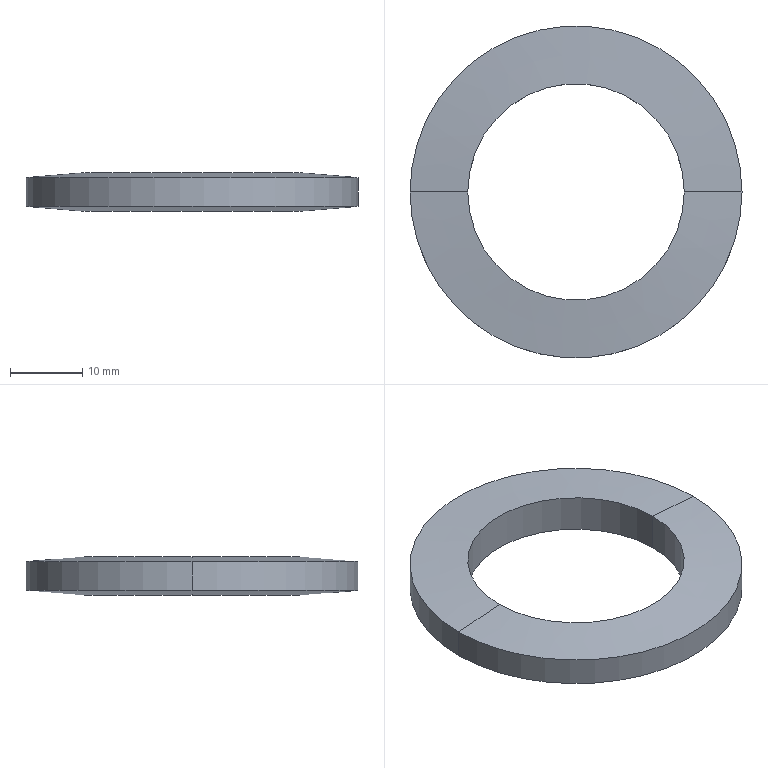Part | SolidWorks | features MBimport 1 | 1 solid | 8 faces | box 46 x 46 x 5.333 mm | volume 4412 mm3 | cone 4 | cylinder 4 | commonest cylinder face diameters 30 x2 46 x2
STEP:
#1=CARTESIAN_POINT('',(-15.,0.,0.08333));
#2=VERTEX_POINT('',#1);
#3=CARTESIAN_POINT('',(15.,0.,0.08333));
#4=VERTEX_POINT('',#3);
#5=CARTESIAN_POINT('',(0.,0.,0.08333));
#6=DIRECTION('',(0.,0.,-1.));
#7=DIRECTION('',(1.,0.,0.));
#8=AXIS2_PLACEMENT_3D('',#5,#6,#7);
#9=CIRCLE('',#8,15.);
#10=EDGE_CURVE('',#2,#4,#9,.T.);
#11=ORIENTED_EDGE('',*,*,#10,.F.);
#12=CARTESIAN_POINT('',(-23.,0.,0.75));
#13=VERTEX_POINT('',#12);
#14=CARTESIAN_POINT('',(-23.,0.,0.75));
#15=DIRECTION('',(-0.9965,0.,0.08305));
#16=VECTOR('',#15,1000.);
#17=LINE('',#14,#16);
#18=EDGE_CURVE('',#2,#13,#17,.T.);
#19=ORIENTED_EDGE('',*,*,#18,.T.);
#20=CARTESIAN_POINT('',(23.,0.,0.75));
#21=VERTEX_POINT('',#20);
#22=CARTESIAN_POINT('',(0.,0.,0.75));
#23=DIRECTION('',(0.,0.,1.));
#24=DIRECTION('',(1.,0.,0.));
#25=AXIS2_PLACEMENT_3D('',#22,#23,#24);
#26=CIRCLE('',#25,23.);
#27=EDGE_CURVE('',#21,#13,#26,.T.);
#28=ORIENTED_EDGE('',*,*,#27,.F.);
#29=CARTESIAN_POINT('',(23.,0.,0.75));
#30=DIRECTION('',(0.9965,0.,0.08305));
#31=VECTOR('',#30,1000.);
#32=LINE('',#29,#31);
#33=EDGE_CURVE('',#4,#21,#32,.T.);
#34=ORIENTED_EDGE('',*,*,#33,.F.);
#35=EDGE_LOOP('',(#11,#19,#28,#34));
#36=FACE_OUTER_BOUND('',#35,.T.);
#37=CARTESIAN_POINT('',(0.,0.,0.75));
#38=DIRECTION('',(0.,0.,1.));
#39=DIRECTION('',(1.,0.,0.));
#40=AXIS2_PLACEMENT_3D('',#37,#38,#39);
#41=CONICAL_SURFACE('',#40,23.,1.488);
#42=ADVANCED_FACE('',(#36),#41,.T.);
#43=CARTESIAN_POINT('',(15.,0.,5.417));
#44=VERTEX_POINT('',#43);
#45=CARTESIAN_POINT('',(-15.,0.,5.417));
#46=VERTEX_POINT('',#45);
#47=CARTESIAN_POINT('',(0.,0.,5.417));
#48=DIRECTION('',(0.,0.,1.));
#49=DIRECTION('',(-1.,0.,0.));
#50=AXIS2_PLACEMENT_3D('',#47,#48,#49);
#51=CIRCLE('',#50,15.);
#52=EDGE_CURVE('',#44,#46,#51,.T.);
#53=ORIENTED_EDGE('',*,*,#52,.F.);
#54=CARTESIAN_POINT('',(23.,0.,4.75));
#55=VERTEX_POINT('',#54);
#56=CARTESIAN_POINT('',(14.,0.,5.5));
#57=DIRECTION('',(0.9965,0.,-0.08305));
#58=VECTOR('',#57,1000.);
#59=LINE('',#56,#58);
#60=EDGE_CURVE('',#44,#55,#59,.T.);
#61=ORIENTED_EDGE('',*,*,#60,.T.);
#62=CARTESIAN_POINT('',(-23.,0.,4.75));
#63=VERTEX_POINT('',#62);
#64=CARTESIAN_POINT('',(0.,0.,4.75));
#65=DIRECTION('',(0.,0.,-1.));
#66=DIRECTION('',(1.,0.,0.));
#67=AXIS2_PLACEMENT_3D('',#64,#65,#66);
#68=CIRCLE('',#67,23.);
#69=EDGE_CURVE('',#63,#55,#68,.T.);
#70=ORIENTED_EDGE('',*,*,#69,.F.);
#71=CARTESIAN_POINT('',(-14.,0.,5.5));
#72=DIRECTION('',(-0.9965,0.,-0.08305));
#73=VECTOR('',#72,1000.);
#74=LINE('',#71,#73);
#75=EDGE_CURVE('',#46,#63,#74,.T.);
#76=ORIENTED_EDGE('',*,*,#75,.F.);
#77=EDGE_LOOP('',(#53,#61,#70,#76));
#78=FACE_OUTER_BOUND('',#77,.T.);
#79=CARTESIAN_POINT('',(0.,0.,5.5));
#80=DIRECTION('',(0.,0.,-1.));
#81=DIRECTION('',(-1.,0.,0.));
#82=AXIS2_PLACEMENT_3D('',#79,#80,#81);
#83=CONICAL_SURFACE('',#82,14.,1.488);
#84=ADVANCED_FACE('',(#78),#83,.T.);
#85=CARTESIAN_POINT('',(0.,0.,5.417));
#86=DIRECTION('',(0.,0.,1.));
#87=DIRECTION('',(-1.,0.,0.));
#88=AXIS2_PLACEMENT_3D('',#85,#86,#87);
#89=CIRCLE('',#88,15.);
#90=EDGE_CURVE('',#46,#44,#89,.T.);
#91=ORIENTED_EDGE('',*,*,#90,.T.);
#92=CARTESIAN_POINT('',(15.,0.,5.5));
#93=DIRECTION('',(0.,0.,-1.));
#94=VECTOR('',#93,1000.);
#95=LINE('',#92,#94);
#96=EDGE_CURVE('',#44,#4,#95,.T.);
#97=ORIENTED_EDGE('',*,*,#96,.T.);
#98=CARTESIAN_POINT('',(0.,0.,0.08333));
#99=DIRECTION('',(0.,0.,-1.));
#100=DIRECTION('',(1.,0.,0.));
#101=AXIS2_PLACEMENT_3D('',#98,#99,#100);
#102=CIRCLE('',#101,15.);
#103=EDGE_CURVE('',#4,#2,#102,.T.);
#104=ORIENTED_EDGE('',*,*,#103,.T.);
#105=CARTESIAN_POINT('',(-15.,0.,5.5));
#106=DIRECTION('',(0.,0.,-1.));
#107=VECTOR('',#106,1000.);
#108=LINE('',#105,#107);
#109=EDGE_CURVE('',#46,#2,#108,.T.);
#110=ORIENTED_EDGE('',*,*,#109,.F.);
#111=EDGE_LOOP('',(#91,#97,#104,#110));
#112=FACE_OUTER_BOUND('',#111,.T.);
#113=CARTESIAN_POINT('',(0.,0.,5.5));
#114=DIRECTION('',(0.,0.,-1.));
#115=DIRECTION('',(-1.,0.,0.));
#116=AXIS2_PLACEMENT_3D('',#113,#114,#115);
#117=CYLINDRICAL_SURFACE('',#116,15.);
#118=ADVANCED_FACE('',(#112),#117,.F.);
#119=ORIENTED_EDGE('',*,*,#69,.T.);
#120=CARTESIAN_POINT('',(23.,0.,5.5));
#121=DIRECTION('',(0.,0.,-1.));
#122=VECTOR('',#121,1000.);
#123=LINE('',#120,#122);
#124=EDGE_CURVE('',#55,#21,#123,.T.);
#125=ORIENTED_EDGE('',*,*,#124,.T.);
#126=ORIENTED_EDGE('',*,*,#27,.T.);
#127=CARTESIAN_POINT('',(-23.,0.,5.5));
#128=DIRECTION('',(0.,0.,-1.));
#129=VECTOR('',#128,1000.);
#130=LINE('',#127,#129);
#131=EDGE_CURVE('',#63,#13,#130,.T.);
#132=ORIENTED_EDGE('',*,*,#131,.F.);
#133=EDGE_LOOP('',(#119,#125,#126,#132));
#134=FACE_OUTER_BOUND('',#133,.T.);
#135=CARTESIAN_POINT('',(0.,0.,5.5));
#136=DIRECTION('',(0.,0.,-1.));
#137=DIRECTION('',(-1.,0.,0.));
#138=AXIS2_PLACEMENT_3D('',#135,#136,#137);
#139=CYLINDRICAL_SURFACE('',#138,23.);
#140=ADVANCED_FACE('',(#134),#139,.T.);
#141=ORIENTED_EDGE('',*,*,#124,.F.);
#142=CARTESIAN_POINT('',(0.,0.,4.75));
#143=DIRECTION('',(0.,0.,-1.));
#144=DIRECTION('',(1.,0.,0.));
#145=AXIS2_PLACEMENT_3D('',#142,#143,#144);
#146=CIRCLE('',#145,23.);
#147=EDGE_CURVE('',#55,#63,#146,.T.);
#148=ORIENTED_EDGE('',*,*,#147,.T.);
#149=ORIENTED_EDGE('',*,*,#131,.T.);
#150=CARTESIAN_POINT('',(0.,0.,0.75));
#151=DIRECTION('',(0.,0.,1.));
#152=DIRECTION('',(1.,0.,0.));
#153=AXIS2_PLACEMENT_3D('',#150,#151,#152);
#154=CIRCLE('',#153,23.);
#155=EDGE_CURVE('',#13,#21,#154,.T.);
#156=ORIENTED_EDGE('',*,*,#155,.T.);
#157=EDGE_LOOP('',(#141,#148,#149,#156));
#158=FACE_OUTER_BOUND('',#157,.T.);
#159=CARTESIAN_POINT('',(0.,0.,5.5));
#160=DIRECTION('',(0.,0.,-1.));
#161=DIRECTION('',(-1.,0.,0.));
#162=AXIS2_PLACEMENT_3D('',#159,#160,#161);
#163=CYLINDRICAL_SURFACE('',#162,23.);
#164=ADVANCED_FACE('',(#158),#163,.T.);
#165=ORIENTED_EDGE('',*,*,#96,.F.);
#166=ORIENTED_EDGE('',*,*,#52,.T.);
#167=ORIENTED_EDGE('',*,*,#109,.T.);
#168=ORIENTED_EDGE('',*,*,#10,.T.);
#169=EDGE_LOOP('',(#165,#166,#167,#168));
#170=FACE_OUTER_BOUND('',#169,.T.);
#171=CARTESIAN_POINT('',(0.,0.,5.5));
#172=DIRECTION('',(0.,0.,-1.));
#173=DIRECTION('',(-1.,0.,0.));
#174=AXIS2_PLACEMENT_3D('',#171,#172,#173);
#175=CYLINDRICAL_SURFACE('',#174,15.);
#176=ADVANCED_FACE('',(#170),#175,.F.);
#177=ORIENTED_EDGE('',*,*,#60,.F.);
#178=ORIENTED_EDGE('',*,*,#90,.F.);
#179=ORIENTED_EDGE('',*,*,#75,.T.);
#180=ORIENTED_EDGE('',*,*,#147,.F.);
#181=EDGE_LOOP('',(#177,#178,#179,#180));
#182=FACE_OUTER_BOUND('',#181,.T.);
#183=CARTESIAN_POINT('',(0.,0.,5.5));
#184=DIRECTION('',(0.,0.,-1.));
#185=DIRECTION('',(-1.,0.,0.));
#186=AXIS2_PLACEMENT_3D('',#183,#184,#185);
#187=CONICAL_SURFACE('',#186,14.,1.488);
#188=ADVANCED_FACE('',(#182),#187,.T.);
#189=ORIENTED_EDGE('',*,*,#18,.F.);
#190=ORIENTED_EDGE('',*,*,#103,.F.);
#191=ORIENTED_EDGE('',*,*,#33,.T.);
#192=ORIENTED_EDGE('',*,*,#155,.F.);
#193=EDGE_LOOP('',(#189,#190,#191,#192));
#194=FACE_OUTER_BOUND('',#193,.T.);
#195=CARTESIAN_POINT('',(0.,0.,0.75));
#196=DIRECTION('',(0.,0.,1.));
#197=DIRECTION('',(1.,0.,0.));
#198=AXIS2_PLACEMENT_3D('',#195,#196,#197);
#199=CONICAL_SURFACE('',#198,23.,1.488);
#200=ADVANCED_FACE('',(#194),#199,.T.);
#201=CLOSED_SHELL('',(#42,#84,#118,#140,#164,#176,#188,#200));
#202=MANIFOLD_SOLID_BREP('',#201);
#203=CARTESIAN_POINT('',(0.,0.,0.));
#204=DIRECTION('',(0.,0.,1.));
#205=DIRECTION('',(1.,0.,0.));
#206=AXIS2_PLACEMENT_3D('',#203,#204,#205);
#207=(LENGTH_UNIT()NAMED_UNIT(*)SI_UNIT(.MILLI.,.METRE.));
#208=UNCERTAINTY_MEASURE_WITH_UNIT(LENGTH_MEASURE(0.00001),#207,'','');
#209=(NAMED_UNIT(*)PLANE_ANGLE_UNIT()SI_UNIT($,.RADIAN.));
#210=(NAMED_UNIT(*)SI_UNIT($,.STERADIAN.)SOLID_ANGLE_UNIT());
#211=(GEOMETRIC_REPRESENTATION_CONTEXT(3)GLOBAL_UNCERTAINTY_ASSIGNED_CONTEXT((#208))GLOBAL_UNIT_ASSIGNED_CONTEXT((#207,#209,#210))REPRESENTATION_CONTEXT('',''));
#212=ADVANCED_BREP_SHAPE_REPRESENTATION('',(#202,#206),#211);